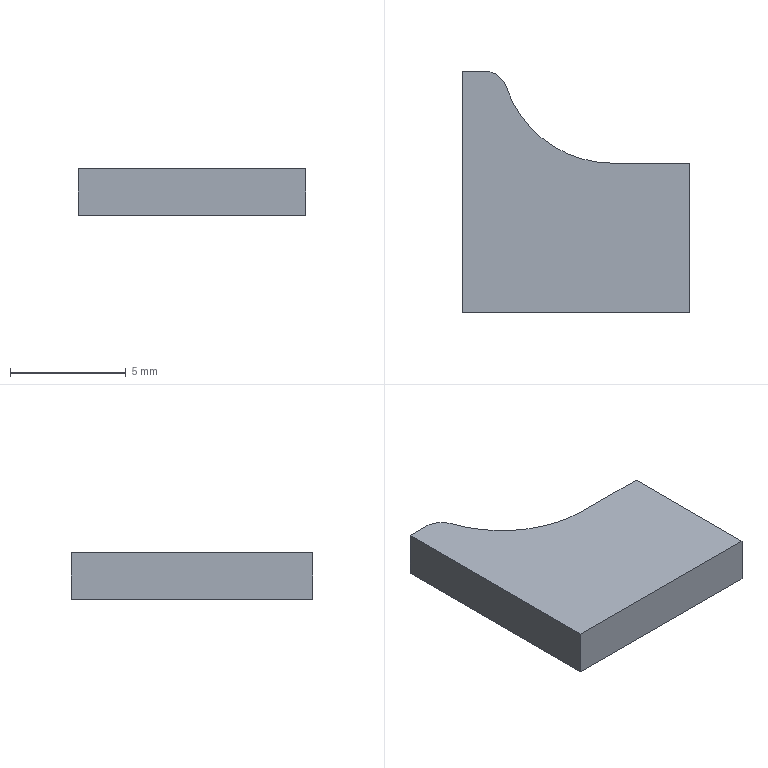Part | SolidWorks | features Cut 2, Fillet 2, ICE 2, BaseBody 1 | 1 solid | 9 faces | box 9.85 x 10.458 x 2 mm | volume 150.551 mm3 | plane 7 | cylinder 2 | commonest cylinder face diameters 2 x1 9.724 x1
STEP:
#1=CARTESIAN_POINT('',(-121.035,209.211,179.684));
#2=VERTEX_POINT('',#1);
#3=CARTESIAN_POINT('',(-121.035,209.211,181.684));
#4=VERTEX_POINT('',#3);
#5=CARTESIAN_POINT('',(-121.035,209.211,174.184));
#6=DIRECTION('',(0.,0.,1.));
#7=VECTOR('',#6,1000.);
#8=LINE('',#5,#7);
#9=EDGE_CURVE('',#2,#4,#8,.T.);
#10=ORIENTED_EDGE('',*,*,#9,.T.);
#11=CARTESIAN_POINT('',(-121.035,202.738,181.684));
#12=VERTEX_POINT('',#11);
#13=CARTESIAN_POINT('',(-121.035,210.238,181.684));
#14=DIRECTION('',(0.,1.,0.));
#15=VECTOR('',#14,1000.);
#16=LINE('',#13,#15);
#17=EDGE_CURVE('',#12,#4,#16,.T.);
#18=ORIENTED_EDGE('',*,*,#17,.F.);
#19=CARTESIAN_POINT('',(-121.035,202.738,179.684));
#20=VERTEX_POINT('',#19);
#21=CARTESIAN_POINT('',(-121.035,202.738,181.684));
#22=DIRECTION('',(0.,0.,1.));
#23=VECTOR('',#22,1000.);
#24=LINE('',#21,#23);
#25=EDGE_CURVE('',#20,#12,#24,.T.);
#26=ORIENTED_EDGE('',*,*,#25,.F.);
#27=CARTESIAN_POINT('',(-121.035,210.238,179.684));
#28=DIRECTION('',(0.,1.,0.));
#29=VECTOR('',#28,1000.);
#30=LINE('',#27,#29);
#31=EDGE_CURVE('',#20,#2,#30,.T.);
#32=ORIENTED_EDGE('',*,*,#31,.T.);
#33=EDGE_LOOP('',(#10,#18,#26,#32));
#34=FACE_OUTER_BOUND('',#33,.T.);
#35=CARTESIAN_POINT('',(-121.035,210.238,181.684));
#36=DIRECTION('',(-1.,0.,0.));
#37=DIRECTION('',(0.,0.,1.));
#38=AXIS2_PLACEMENT_3D('',#35,#36,#37);
#39=PLANE('',#38);
#40=ADVANCED_FACE('',(#34),#39,.F.);
#41=CARTESIAN_POINT('',(-128.981,212.516,181.684));
#42=VERTEX_POINT('',#41);
#43=CARTESIAN_POINT('',(-124.375,209.211,181.684));
#44=VERTEX_POINT('',#43);
#45=CARTESIAN_POINT('',(-124.375,214.073,181.684));
#46=DIRECTION('',(0.,0.,1.));
#47=DIRECTION('',(1.,0.,0.));
#48=AXIS2_PLACEMENT_3D('',#45,#46,#47);
#49=CIRCLE('',#48,4.862);
#50=EDGE_CURVE('',#42,#44,#49,.T.);
#51=ORIENTED_EDGE('',*,*,#50,.F.);
#52=CARTESIAN_POINT('',(-129.928,213.196,181.684));
#53=VERTEX_POINT('',#52);
#54=CARTESIAN_POINT('',(-129.928,212.196,181.684));
#55=DIRECTION('',(0.,0.,1.));
#56=DIRECTION('',(-1.,0.,0.));
#57=AXIS2_PLACEMENT_3D('',#54,#55,#56);
#58=CIRCLE('',#57,1.);
#59=EDGE_CURVE('',#42,#53,#58,.T.);
#60=ORIENTED_EDGE('',*,*,#59,.T.);
#61=CARTESIAN_POINT('',(-130.885,213.196,181.684));
#62=VERTEX_POINT('',#61);
#63=CARTESIAN_POINT('',(-133.334,213.196,181.684));
#64=DIRECTION('',(1.,0.,0.));
#65=VECTOR('',#64,1000.);
#66=LINE('',#63,#65);
#67=EDGE_CURVE('',#62,#53,#66,.T.);
#68=ORIENTED_EDGE('',*,*,#67,.F.);
#69=CARTESIAN_POINT('',(-130.885,202.738,181.684));
#70=VERTEX_POINT('',#69);
#71=CARTESIAN_POINT('',(-130.885,217.898,181.684));
#72=DIRECTION('',(0.,-1.,0.));
#73=VECTOR('',#72,1000.);
#74=LINE('',#71,#73);
#75=EDGE_CURVE('',#62,#70,#74,.T.);
#76=ORIENTED_EDGE('',*,*,#75,.T.);
#77=CARTESIAN_POINT('',(-130.885,202.738,181.684));
#78=DIRECTION('',(-1.,0.,0.));
#79=VECTOR('',#78,1000.);
#80=LINE('',#77,#79);
#81=EDGE_CURVE('',#12,#70,#80,.T.);
#82=ORIENTED_EDGE('',*,*,#81,.F.);
#83=ORIENTED_EDGE('',*,*,#17,.T.);
#84=CARTESIAN_POINT('',(0.,209.211,181.684));
#85=DIRECTION('',(-1.,0.,0.));
#86=VECTOR('',#85,1000.);
#87=LINE('',#84,#86);
#88=EDGE_CURVE('',#4,#44,#87,.T.);
#89=ORIENTED_EDGE('',*,*,#88,.T.);
#90=EDGE_LOOP('',(#51,#60,#68,#76,#82,#83,#89));
#91=FACE_OUTER_BOUND('',#90,.T.);
#92=CARTESIAN_POINT('',(-117.673,229.287,181.684));
#93=DIRECTION('',(0.,0.,-1.));
#94=DIRECTION('',(-1.,0.,0.));
#95=AXIS2_PLACEMENT_3D('',#92,#93,#94);
#96=PLANE('',#95);
#97=ADVANCED_FACE('',(#91),#96,.F.);
#98=CARTESIAN_POINT('',(-130.885,213.196,179.684));
#99=VERTEX_POINT('',#98);
#100=CARTESIAN_POINT('',(-129.928,213.196,179.684));
#101=VERTEX_POINT('',#100);
#102=CARTESIAN_POINT('',(-133.334,213.196,179.684));
#103=DIRECTION('',(1.,0.,0.));
#104=VECTOR('',#103,1000.);
#105=LINE('',#102,#104);
#106=EDGE_CURVE('',#99,#101,#105,.T.);
#107=ORIENTED_EDGE('',*,*,#106,.T.);
#108=CARTESIAN_POINT('',(-128.981,212.516,179.684));
#109=VERTEX_POINT('',#108);
#110=CARTESIAN_POINT('',(-129.928,212.196,179.684));
#111=DIRECTION('',(0.,0.,-1.));
#112=DIRECTION('',(-1.,0.,0.));
#113=AXIS2_PLACEMENT_3D('',#110,#111,#112);
#114=CIRCLE('',#113,1.);
#115=EDGE_CURVE('',#101,#109,#114,.T.);
#116=ORIENTED_EDGE('',*,*,#115,.T.);
#117=CARTESIAN_POINT('',(-124.375,209.211,179.684));
#118=VERTEX_POINT('',#117);
#119=CARTESIAN_POINT('',(-124.375,214.073,179.684));
#120=DIRECTION('',(0.,0.,-1.));
#121=DIRECTION('',(-1.,0.,0.));
#122=AXIS2_PLACEMENT_3D('',#119,#120,#121);
#123=CIRCLE('',#122,4.862);
#124=EDGE_CURVE('',#118,#109,#123,.T.);
#125=ORIENTED_EDGE('',*,*,#124,.F.);
#126=CARTESIAN_POINT('',(-117.673,209.211,179.684));
#127=DIRECTION('',(1.,0.,0.));
#128=VECTOR('',#127,1000.);
#129=LINE('',#126,#128);
#130=EDGE_CURVE('',#118,#2,#129,.T.);
#131=ORIENTED_EDGE('',*,*,#130,.T.);
#132=ORIENTED_EDGE('',*,*,#31,.F.);
#133=CARTESIAN_POINT('',(-130.885,202.738,179.684));
#134=VERTEX_POINT('',#133);
#135=CARTESIAN_POINT('',(-130.885,202.738,179.684));
#136=DIRECTION('',(1.,0.,0.));
#137=VECTOR('',#136,1000.);
#138=LINE('',#135,#137);
#139=EDGE_CURVE('',#134,#20,#138,.T.);
#140=ORIENTED_EDGE('',*,*,#139,.F.);
#141=CARTESIAN_POINT('',(-130.885,217.898,179.684));
#142=DIRECTION('',(0.,-1.,0.));
#143=VECTOR('',#142,1000.);
#144=LINE('',#141,#143);
#145=EDGE_CURVE('',#99,#134,#144,.T.);
#146=ORIENTED_EDGE('',*,*,#145,.F.);
#147=EDGE_LOOP('',(#107,#116,#125,#131,#132,#140,#146));
#148=FACE_OUTER_BOUND('',#147,.T.);
#149=CARTESIAN_POINT('',(-117.673,229.287,179.684));
#150=DIRECTION('',(0.,0.,-1.));
#151=DIRECTION('',(-1.,0.,0.));
#152=AXIS2_PLACEMENT_3D('',#149,#150,#151);
#153=PLANE('',#152);
#154=ADVANCED_FACE('',(#148),#153,.T.);
#155=ORIENTED_EDGE('',*,*,#75,.F.);
#156=CARTESIAN_POINT('',(-130.885,213.196,181.684));
#157=DIRECTION('',(0.,0.,-1.));
#158=VECTOR('',#157,1000.);
#159=LINE('',#156,#158);
#160=EDGE_CURVE('',#62,#99,#159,.T.);
#161=ORIENTED_EDGE('',*,*,#160,.T.);
#162=ORIENTED_EDGE('',*,*,#145,.T.);
#163=CARTESIAN_POINT('',(-130.885,202.738,181.684));
#164=DIRECTION('',(0.,0.,-1.));
#165=VECTOR('',#164,1000.);
#166=LINE('',#163,#165);
#167=EDGE_CURVE('',#70,#134,#166,.T.);
#168=ORIENTED_EDGE('',*,*,#167,.F.);
#169=EDGE_LOOP('',(#155,#161,#162,#168));
#170=FACE_OUTER_BOUND('',#169,.T.);
#171=CARTESIAN_POINT('',(-130.885,217.898,181.684));
#172=DIRECTION('',(1.,0.,0.));
#173=DIRECTION('',(0.,0.,-1.));
#174=AXIS2_PLACEMENT_3D('',#171,#172,#173);
#175=PLANE('',#174);
#176=ADVANCED_FACE('',(#170),#175,.F.);
#177=ORIENTED_EDGE('',*,*,#167,.T.);
#178=ORIENTED_EDGE('',*,*,#139,.T.);
#179=ORIENTED_EDGE('',*,*,#25,.T.);
#180=ORIENTED_EDGE('',*,*,#81,.T.);
#181=EDGE_LOOP('',(#177,#178,#179,#180));
#182=FACE_OUTER_BOUND('',#181,.T.);
#183=CARTESIAN_POINT('',(0.,202.738,0.));
#184=DIRECTION('',(0.,-1.,0.));
#185=DIRECTION('',(0.,0.,-1.));
#186=AXIS2_PLACEMENT_3D('',#183,#184,#185);
#187=PLANE('',#186);
#188=ADVANCED_FACE('',(#182),#187,.T.);
#189=CARTESIAN_POINT('',(-124.375,209.211,174.184));
#190=DIRECTION('',(0.,0.,1.));
#191=VECTOR('',#190,1000.);
#192=LINE('',#189,#191);
#193=EDGE_CURVE('',#118,#44,#192,.T.);
#194=ORIENTED_EDGE('',*,*,#193,.T.);
#195=ORIENTED_EDGE('',*,*,#88,.F.);
#196=ORIENTED_EDGE('',*,*,#9,.F.);
#197=ORIENTED_EDGE('',*,*,#130,.F.);
#198=EDGE_LOOP('',(#194,#195,#196,#197));
#199=FACE_OUTER_BOUND('',#198,.T.);
#200=CARTESIAN_POINT('',(0.,209.211,174.184));
#201=DIRECTION('',(0.,1.,0.));
#202=DIRECTION('',(0.,0.,1.));
#203=AXIS2_PLACEMENT_3D('',#200,#201,#202);
#204=PLANE('',#203);
#205=ADVANCED_FACE('',(#199),#204,.T.);
#206=ORIENTED_EDGE('',*,*,#124,.T.);
#207=CARTESIAN_POINT('',(-128.981,212.516,174.184));
#208=DIRECTION('',(0.,0.,1.));
#209=VECTOR('',#208,1000.);
#210=LINE('',#207,#209);
#211=EDGE_CURVE('',#109,#42,#210,.T.);
#212=ORIENTED_EDGE('',*,*,#211,.T.);
#213=ORIENTED_EDGE('',*,*,#50,.T.);
#214=ORIENTED_EDGE('',*,*,#193,.F.);
#215=EDGE_LOOP('',(#206,#212,#213,#214));
#216=FACE_OUTER_BOUND('',#215,.T.);
#217=CARTESIAN_POINT('',(-124.375,214.073,174.184));
#218=DIRECTION('',(0.,0.,1.));
#219=DIRECTION('',(1.,0.,0.));
#220=AXIS2_PLACEMENT_3D('',#217,#218,#219);
#221=CYLINDRICAL_SURFACE('',#220,4.862);
#222=ADVANCED_FACE('',(#216),#221,.F.);
#223=ORIENTED_EDGE('',*,*,#67,.T.);
#224=CARTESIAN_POINT('',(-129.928,213.196,179.684));
#225=DIRECTION('',(0.,0.,-1.));
#226=VECTOR('',#225,1000.);
#227=LINE('',#224,#226);
#228=EDGE_CURVE('',#53,#101,#227,.T.);
#229=ORIENTED_EDGE('',*,*,#228,.T.);
#230=ORIENTED_EDGE('',*,*,#106,.F.);
#231=ORIENTED_EDGE('',*,*,#160,.F.);
#232=EDGE_LOOP('',(#223,#229,#230,#231));
#233=FACE_OUTER_BOUND('',#232,.T.);
#234=CARTESIAN_POINT('',(-133.334,213.196,179.684));
#235=DIRECTION('',(0.,-1.,0.));
#236=DIRECTION('',(0.,0.,-1.));
#237=AXIS2_PLACEMENT_3D('',#234,#235,#236);
#238=PLANE('',#237);
#239=ADVANCED_FACE('',(#233),#238,.F.);
#240=ORIENTED_EDGE('',*,*,#115,.F.);
#241=ORIENTED_EDGE('',*,*,#228,.F.);
#242=ORIENTED_EDGE('',*,*,#59,.F.);
#243=ORIENTED_EDGE('',*,*,#211,.F.);
#244=EDGE_LOOP('',(#240,#241,#242,#243));
#245=FACE_OUTER_BOUND('',#244,.T.);
#246=CARTESIAN_POINT('',(-129.928,212.196,174.184));
#247=DIRECTION('',(0.,0.,1.));
#248=DIRECTION('',(1.,0.,0.));
#249=AXIS2_PLACEMENT_3D('',#246,#247,#248);
#250=CYLINDRICAL_SURFACE('',#249,1.);
#251=ADVANCED_FACE('',(#245),#250,.T.);
#252=CLOSED_SHELL('',(#40,#97,#154,#176,#188,#205,#222,#239,#251));
#253=MANIFOLD_SOLID_BREP('',#252);
#254=CARTESIAN_POINT('',(0.,0.,0.));
#255=DIRECTION('',(0.,0.,1.));
#256=DIRECTION('',(1.,0.,0.));
#257=AXIS2_PLACEMENT_3D('',#254,#255,#256);
#258=(LENGTH_UNIT()NAMED_UNIT(*)SI_UNIT(.MILLI.,.METRE.));
#259=UNCERTAINTY_MEASURE_WITH_UNIT(LENGTH_MEASURE(0.00001),#258,'','');
#260=(NAMED_UNIT(*)PLANE_ANGLE_UNIT()SI_UNIT($,.RADIAN.));
#261=(NAMED_UNIT(*)SI_UNIT($,.STERADIAN.)SOLID_ANGLE_UNIT());
#262=(GEOMETRIC_REPRESENTATION_CONTEXT(3)GLOBAL_UNCERTAINTY_ASSIGNED_CONTEXT((#259))GLOBAL_UNIT_ASSIGNED_CONTEXT((#258,#260,#261))REPRESENTATION_CONTEXT('',''));
#263=ADVANCED_BREP_SHAPE_REPRESENTATION('',(#253,#257),#262);